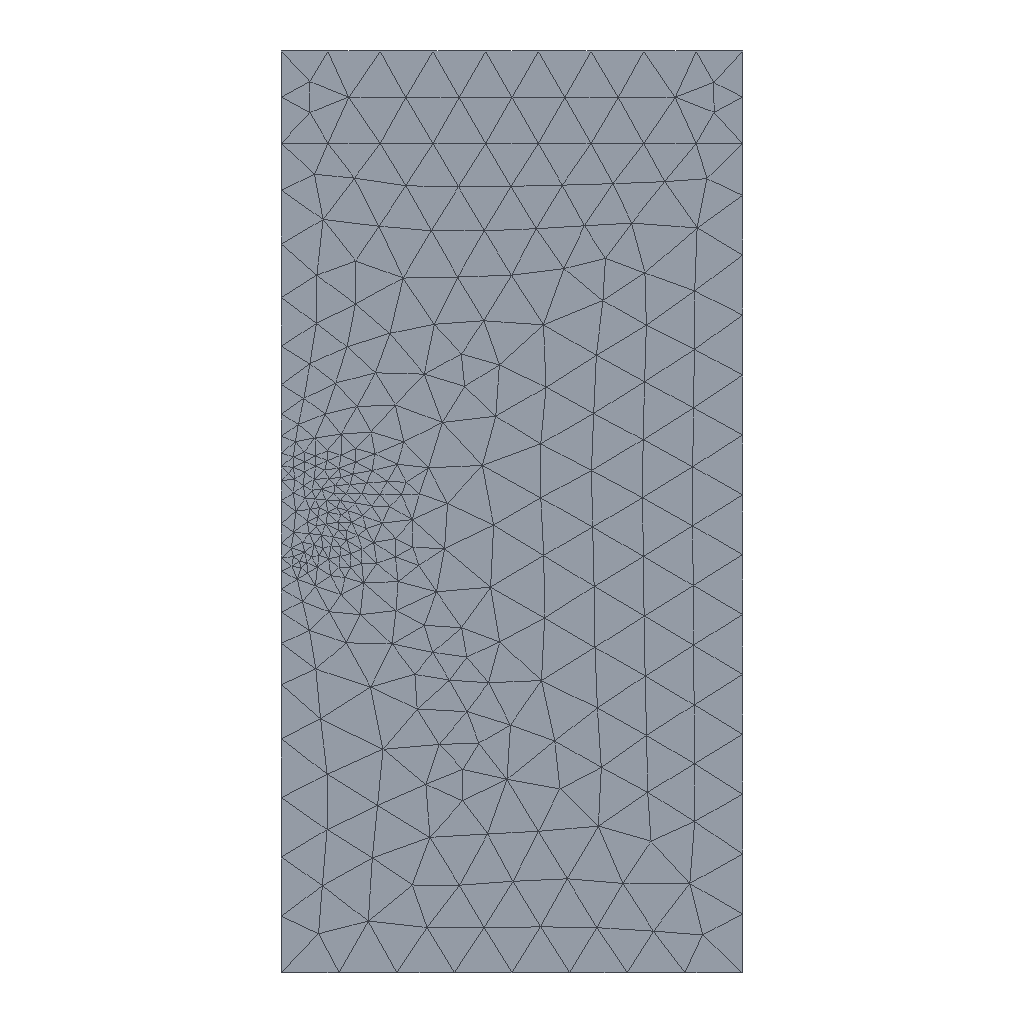Simulation study | comsol
Notes in the study folder:
k_liver 0.56[W/(m*K)] Thermal conductivity liver
rho_blood 1e3[kg/m^3] Density blood
Cp_blood 3639[J/(kg*K)] Heat capacity blood
omega_blood 3.6e-3[1/s] Blood perfusion rate
T_blood 37[degC] Temperature blood
P_in 10[W] Microwave power input
f 2.45[GHz] Microwave frequency
eps_diel 2.6[1] Dielectric relative permittivity
eps_cat 2.6[1] Catheter relative permittivity
eps_liver 43.03[1] Liver relative permittivity
sigma_liver 1.69[S/m] Conductivity liver
rho_liver 1038[kg/m^3] Liver density
Cp_liver 4187[J/(kg*K)] Liver heat capacity
sigma_cat 1e-6[S/m] Catheter conductivity
mur_cat 1[1] Catheter relative permeability
k_ptfe 0.25[W/(m*K)] Thermal conductivity PTFE
rho_ptfe 2200[kg/m^3] Density PTFE
Cp_ptfe 1300[J/(kg*K)] PTFE heat capacity
sigma_diel 1e-6[S/m] Microwave center feed
mur_diel 1[1] Relative permeability dielectric
mur_liver 1[1] Relative permeability liver
Set-up summary:
category,name,step,type,value,unit,region
solver,comsol,,COMSOL Multiphysics 6.4 (Build: 293)
units,SI; geometry length unit m,,stated,COMSOL default unit system (SI)
analysis,Study 1,,Transient,space_dimension=2D
load_step,std1/time,std1/time,Transient,"type=Transient; times=range(0,10,600)"
mesh,nodes,,,330
mesh,elements,,,599
element_type,tri,,,599
element_type,edg,,,80
element_type,vtx,,,9
component,mod1,,2D,geometry=geom1; domains=3
physics,Heat Transfer (ht),mod1,BioHeat,"T(T), discontinuousdamagedtissueindicator(discontinuousdamagedtissueindicator), continuousdamagedtissueindicator(continuousdamagedtissueindicator), thermaldamageindicator(thermaldamageindicator), radiativeintensity(radiativeintensity), incidentradiation(incidentradiation), surfaceradiosity(surfaceradiosity)"
parameter,rho_blood,,,1000[kg/m^3]
parameter,C_blood,,,4200[J/(kg*K)]
parameter,T_blood,,,37[degC]
parameter,k_skin,,,0.2[W/(m*K)]
parameter,rho_skin,,,1200[kg/m^3]
parameter,C_skin,,,3600[J/(kg*K)]
parameter,wb_skin,,,3e-3[1/s]
parameter,k_tissue,,,0.5[W/(m*K)]
parameter,rho_tissue,,,1050[kg/m^3]
parameter,C_tissue,,,3600[J/(kg*K)]
parameter,wb_tissue,,,6e-3[1/s]
parameter,k_tumor,,,0.5[W/(m*K)]
parameter,rho_tumor,,,1050[kg/m^3]
parameter,C_tumor,,,3600[J/(kg*K)]
parameter,wb_tumor,,,6e-3[1/s]
parameter,Q_met,,,400[W/m^3]
parameter,T0,,,37[degC]
parameter,h_conv,,,10[W/(m^2*K)]
parameter,T_inf,,,10[degC]
parameter,I0,,,1.4[W/mm^2]
parameter,sigma,,,5[mm]
bc,Biological Tissue 1 (bt1),mod1/ht,BiologicalTissue,k=k_skin; rho=rho_skin; Cp=C_skin; streamline=0; crosswind=0; pref=1[atm]; hasPhaseChange=0; Solid_material=dommat; u_prime=0 0 0; dfltopaque=1; thermalConductivityModel=Standard,,selection [3]
bc,Axial Symmetry 1 (axi1),mod1/ht,AxialSymmetry,,,"selection [1, 3, 4, 5]"
bc,Thermal Insulation 1 (ins1),mod1/ht,ThermalInsulation,,,"selection [2, 8, 9]"
bc,Initial Values 1 (init1),mod1/ht,init,Tinit=T0; Tinit_resistive=293.15[K],,"selection [1, 2, 3]"
bc,Continuity (dcont1),mod1/ht,Continuity,pairDisconnect=1; pairSelection=all; pairsList=0,,selection []
bc,Biological Tissue 2 (bt2),mod1/ht,BiologicalTissue,k=k_tissue; rho=rho_tissue; Cp=C_tissue; streamline=0; crosswind=0; pref=1[atm]; hasPhaseChange=0; Solid_material=dommat; u_prime=0 0 0; dfltopaque=1; thermalConductivityModel=Standard,,selection [1]
bc,Biological Tissue 3 (bt3),mod1/ht,BiologicalTissue,k=k_tumor; rho=rho_tumor; Cp=C_tumor; streamline=0; crosswind=0; pref=1[atm]; hasPhaseChange=0; Solid_material=dommat; u_prime=0 0 0; dfltopaque=1; thermalConductivityModel=Standard,,selection [2]
bc,Heat Source 1 (hs1),mod1/ht,HeatSource,Q0=Q_laser; heatSourceType=GeneralSource; qs=0; P0=0; materialType=solid; harmonicPerturbation=0; loadGroup=default,,"selection [1, 2, 3]"
bc,Heat Flux 1 (hf1),mod1/ht,HeatFluxBoundary,HeatFluxType=ConvectiveHeatFlux; q0_input=0; h=h_conv; Text=T_inf; P0=0; HeatTransferCoefficientType=UserDef; ExtNaturalConvectionType=VerticalWall; IntNaturalConvectionType=NarrowChimneyParallelPlates; ExtForcedConvectionType=PlateAveragedTransferCoefficient; IntForcedConvectionType=IsothermalTube; ExternalFluidType=Air; Lwall=0; Ldia=0; phi_tilt=0; Ldis=0; Hchimn=0; D=0; Dcyl=0; Dsph=0; Dvcyl=0;,,selection [7]
bc,Local Thermal Nonequilibrium Boundary 1 (ltneb1),mod1/ht,LocalThermalNonequilibriumBoundary,,,selection []
COMSOL model file for Java, long lists of numbers shortened:
/*
 * em_deck.java
 */

import com.comsol.model.*;
import com.comsol.model.util.*;

/** Model exported on Oct 28 2026, 08:57 by COMSOL 6.4.0.293. */
public class em_deck {

  public static Model run() {
    Model model = ModelUtil.create("Model");

    model.modelPath("");

    model.modelNode().create("mod1");

    model.geom().create("geom1", 2);
    model.geom("geom1").axisymmetric(true);

    model.mesh().create("mesh1", "geom1");

    model.physics()
         .create("ht", "BioHeat", "geom1", new String[]{"I1", "I2", "I3", "I4", "I5", "I6", "I7", "I8", "I9", "I10",
         "I11", "I12"});

    model.study().create("std1");
    model.study("std1").feature().create("time", "Transient");

    model.param().set("rho_blood", "1000[kg/m^3]");
    model.param().descr("rho_blood", "Density blood");
    model.param().set("C_blood", "4200[J/(kg*K)]");
    model.param().descr("C_blood", "Heat capacity blood");
    model.param().set("T_blood", "37[degC]");
    model.param().descr("T_blood", "Temperature blood");
    model.param().set("k_skin", "0.2[W/(m*K)]");
    model.param().descr("k_skin", "Thermal conductivity skin");
    model.param().set("rho_skin", "1200[kg/m^3]");
    model.param().descr("rho_skin", "Density skin");
    model.param().set("C_skin", "3600[J/(kg*K)]");
    model.param().descr("C_skin", "Heat capacity skin");
    model.param().set("wb_skin", "3e-3[1/s]");
    model.param().descr("wb_skin", "Blood perfusion rate skin");
    model.param().set("k_tissue", "0.5[W/(m*K)]");
    model.param().descr("k_tissue", "Thermal conductivity tissue");
    model.param().set("rho_tissue", "1050[kg/m^3]");
    model.param().descr("rho_tissue", "Density tissue");
    model.param().set("C_tissue", "3600[J/(kg*K)]");
    model.param().descr("C_tissue", "Heat capacity tissue");
    model.param().set("wb_tissue", "6e-3[1/s]");
    model.param().descr("wb_tissue", "Blood perfusion rate tissue");
    model.param().set("k_tumor", "0.5[W/(m*K)]");
    model.param().descr("k_tumor", "Thermal conductivity tumor");
    model.param().set("rho_tumor", "1050[kg/m^3]");
    model.param().descr("rho_tumor", "Density tumor");
    model.param().set("C_tumor", "3600[J/(kg*K)]");
    model.param().descr("C_tumor", "Heat capacity tumor");
    model.param().set("wb_tumor", "6e-3[1/s]");
    model.param().descr("wb_tumor", "Blood perfusion rate tumor");
    model.param().set("Q_met", "400[W/m^3]");
    model.param().descr("Q_met", "Metabolic heat generation");
    model.param().set("T0", "37[degC]");
    model.param().descr("T0", "Temperature reference blood");
    model.param().set("h_conv", "10[W/(m^2*K)]");
    model.param().descr("h_conv", "Heat transfer coefficient skin");
    model.param().set("T_inf", "10[degC]");
    model.param().descr("T_inf", "Temperature domain boundary");
    model.param().set("I0", "1.4[W/mm^2]");
    model.param().descr("I0", "Laser irradiation power");
    model.param().set("sigma", "5[mm]");
    model.param().descr("sigma", "Laser beam width coefficient");

    model.name(".mph");

    model.geom("geom1").feature().create("r1", "Rectangle");
    model.geom("geom1").feature("r1").setIndex("size", "0.1[m]", 0);
    model.geom("geom1").feature("r1").setIndex("size", "0.09[m]", 1);
    model.geom("geom1").feature("r1").setIndex("pos", "-0.05[m]", 0);
    model.geom("geom1").feature("r1").setIndex("pos", "-0.1", 1);
    model.geom("geom1").run("r1");
    model.geom("geom1").run("r1");
    model.geom("geom1").feature().create("r2", "Rectangle");
    model.geom("geom1").feature("r2").setIndex("size", "0.1[m]", 0);
    model.geom("geom1").feature("r2").setIndex("size", "0.01[m]", 1);
    model.geom("geom1").feature("r2").setIndex("pos", "-0.05[m]", 0);
    model.geom("geom1").feature("r2").setIndex("pos", "-0.01[m]", 1);
    model.geom("geom1").run("r2");
    model.geom("geom1").run("r2");
    model.geom("geom1").feature().create("c1", "Circle");
    model.geom("geom1").feature("c1").set("r", "0.005[m]");
    model.geom("geom1").feature("c1").setIndex("pos", "0[m]", 0);
    model.geom("geom1").feature("c1").setIndex("pos", "-0.05[m]", 1);
    model.geom("geom1").runAll();
    model.geom("geom1").run("c1");
    model.geom("geom1").feature().create("r3", "Rectangle");
    model.geom("geom1").feature("r3").setIndex("size", "0.05[m]", 0);
    model.geom("geom1").feature("r3").setIndex("size", "0.1[m]", 1);
    model.geom("geom1").feature("r3").setIndex("pos", "-0.05[m]", 0);
    model.geom("geom1").feature("r3").setIndex("pos", "-0.1[m]", 1);
    model.geom("geom1").run("r3");
    model.geom("geom1").run("r3");
    model.geom("geom1").feature().create("dif1", "Difference");
    model.geom("geom1").feature("dif1").selection("input").set(new String[]{"c1", "r1", "r2"});
    model.geom("geom1").feature("dif1").selection("input2").set(new String[]{"r3"});
    model.geom("geom1").run("dif1");
    model.geom("geom1").run();

    model.variable().create("var1");
    model.variable("var1").model("mod1");
    model.variable("var1").selection().geom("geom1", 2);
    model.variable("var1").selection().global();
    model.variable("var1").selection().geom("geom1", 2);
    model.variable("var1").selection().set(new int[]{1, 3});
    model.variable("var1").set("a", "0.1[1/m]");
    model.variable("var1").descr("a", "Absorptance");
    model.variable("var1").descr("a", "Absorbance");
    model.variable().create("var2");
    model.variable("var2").model("mod1");
    model.variable("var2").selection().geom("geom1", 2);
    model.variable("var2").selection().set(new int[]{2});
    model.variable("var2").set("a", "4[1/m]");
    model.variable("var2").descr("a", "Absorbance");
    model.variable().create("var3");
    model.variable("var3").model("mod1");
    model.variable("var3").set("Q_laser", "I0*a*exp(a*z-r^2/(2*sigma^2))");
    model.variable("var3").descr("Q_laser", "Laser energy distribution");

    model.physics("ht").feature().create("bt2", "BiologicalTissue", 2);
    model.physics("ht").feature().remove("bt2");
    model.physics("ht").feature("bt1").set("k_mat", 1, "userdef");
    model.physics("ht").feature("bt1").set("rho_mat", 1, "userdef");
    model.physics("ht").feature("bt1").set("Cp_mat", 1, "userdef");
    model.physics("ht").feature("bt1").set("Cp", 1, "C_skin");
    model.physics("ht").feature("bt1").set("rho", 1, "rho_skin");
    model.physics("ht").feature("bt1")
         .set("k", new String[]{"k_skin", "0", "0", "0", "k_skin", "0", "0", "0", "k_skin"});
    model.physics("ht").feature().create("bt2", "BiologicalTissue", 2);
    model.physics("ht").feature("bt2").set("k_mat", 1, "userdef");
    model.physics("ht").feature("bt2").set("rho_mat", 1, "userdef");
    model.physics("ht").feature("bt2").set("Cp_mat", 1, "userdef");
    model.physics("ht").feature("bt2")
         .set("k", new String[]{"k_tissue", "0", "0", "0", "k_tissue", "0", "0", "0", "k_tissue"});
    model.physics("ht").feature("bt2").set("rho", 1, "rho_tissue");
    model.physics("ht").feature("bt2").set("Cp", 1, "C_tissue");
    model.physics("ht").feature("bt2").selection().set(new int[]{1});
    model.physics("ht").feature("bt2").feature("bh1").set("rhobl", 1, "rho_blood");
    model.physics("ht").feature("bt2").feature("bh1").set("Cb", 1, "C_blood");
    model.physics("ht").feature("bt2").feature("bh1").set("omegab", 1, "wb_tissue");
    model.physics("ht").feature("bt2").feature("bh1").set("Tb", 1, "T_blood");
    model.physics("ht").feature("bt2").feature("bh1").set("Qmet", 1, "Q_met");
    model.physics("ht").feature().create("bt3", "BiologicalTissue", 2);
    model.physics("ht").feature("bt3").selection().set(new int[]{2});
    model.physics("ht").feature("bt3").set("k_mat", 1, "userdef");
    model.physics("ht").feature("bt3").set("rho_mat", 1, "userdef");
    model.physics("ht").feature("bt3").set("Cp_mat", 1, "userdef");
    model.physics("ht").feature("bt3")
         .set("k", new String[]{"k_tumor", "0", "0", "0", "k_tumor", "0", "0", "0", "k_tumor"});
    model.physics("ht").feature("bt3").set("rho", 1, "rho_tumor");
    model.physics("ht").feature("bt3").set("Cp", 1, "C_tumor");
    model.physics("ht").feature("bt3").feature("bh1").set("rhobl", 1, "rho_blood");
    model.physics("ht").feature("bt3").feature("bh1").set("Cb", 1, "C_blood");
    model.physics("ht").feature("bt3").feature("bh1").set("omegab", 1, "wb_tumor");
    model.physics("ht").feature("bt3").feature("bh1").set("Tb", 1, "T_blood");
    model.physics("ht").feature("bt3").feature("bh1").set("Qmet", 1, "Q_met");

    model.name(".mph");

    model.physics("ht").feature("init1").set("T", 1, "T0");
    model.physics("ht").feature("bt1").feature("bh1").set("rhobl", 1, "rho_blood");
    model.physics("ht").feature("bt1").feature("bh1").set("Cb", 1, "C_blood");
    model.physics("ht").feature("bt1").feature("bh1").set("omegab", 1, "wb_skin");
    model.physics("ht").feature("bt1").feature("bh1").set("Tb", 1, "T_blood");
    model.physics("ht").feature("bt1").feature("bh1").set("Qmet", 1, "Q_met");
    model.physics("ht").feature().create("hs1", "HeatSource", 2);
    model.physics("ht").feature("hs1").selection().all();
    model.physics("ht").feature("hs1").set("Q", 1, "Q_laser");
    model.physics("ht").feature().create("hf1", "HeatFluxBoundary", 1);
    model.physics("ht").feature("hf1").selection().set(new int[]{7});
    model.physics("ht").feature("hf1").set("HeatFluxType", 1, "InwardHeatFlux");
    model.physics("ht").feature("hf1").set("h", 1, "h_conv");
    model.physics("ht").feature("hf1").set("Text", 1, "T_inf");

    model.mesh("mesh1").feature().create("ftri1", "FreeTri");
    model.mesh("mesh1").run();

    model.study("std1").feature("time").set("tlist", "range(0,10,600)");

    model.sol().create("sol1");
    model.sol("sol1").study("std1");
    model.sol("sol1").feature().create("st1", "StudyStep");
    model.sol("sol1").feature("st1").set("study", "std1");
    model.sol("sol1").feature("st1").set("studystep", "time");
    model.sol("sol1").feature().create("v1", "Variables");
    model.sol("sol1").feature().create("t1", "Time");
    model.sol("sol1").feature("t1").set("tlist", "range(0,10,600)");
    model.sol("sol1").feature("t1").set("plot", "off");
    model.sol("sol1").feature("t1").set("plotfreq", "tout");
    model.sol("sol1").feature("t1").set("probesel", "all");
    model.sol("sol1").feature("t1").set("probes", new String[]{});
    model.sol("sol1").feature("t1").set("probefreq", "tsteps");
    model.sol("sol1").feature("t1").set("estrat", "exclude");
    model.sol("sol1").feature("t1").set("maxorder", 2);
    model.sol("sol1").feature("t1").set("control", "time");
    model.sol("sol1").feature("t1").feature().create("fc1", "FullyCoupled");
    model.sol("sol1").feature("t1").feature("fc1").set("jtech", "once");
    model.sol("sol1").feature("t1").feature("fc1").set("maxiter", 5);
    model.sol("sol1").feature("t1").feature().create("d1", "Direct");
    model.sol("sol1").feature("t1").feature("d1").set("linsolver", "pardiso");
    model.sol("sol1").feature("t1").feature("fc1").set("linsolver", "d1");
    model.sol("sol1").feature("t1").feature("fc1").set("jtech", "once");
    model.sol("sol1").feature("t1").feature("fc1").set("maxiter", 5);
    model.sol("sol1").feature("t1").feature().remove("fcDef");
    model.sol("sol1").attach("std1");

    model.result().create("pg1", 2);
    model.result("pg1").set("data", "dset1");
    model.result("pg1").feature().create("surf1", "Surface");
    model.result("pg1").feature("surf1").set("expr", "T");
    model.result("pg1").feature("surf1").set("descr", "Temperature");

    model.sol("sol1").runAll();

    model.result("pg1").set("windowtitle", "Graphics");
    model.result("pg1").run();
    model.result("pg1").run();
    model.result("pg1").feature("surf1").set("unit", "degC");
    model.result("pg1").run();
    model.result("pg1").feature("surf1").set("unit", "K");
    model.result("pg1").run();
    model.result("pg1").feature("surf1").set("unit", "degC");

    model.label("in.mph");

    return model;
  }

  public static void main(String[] args) {
    run();
  }

}
Results summary:
result,max T = abs(mod1.T),dset1 (61 solution(s)),,360.565,K